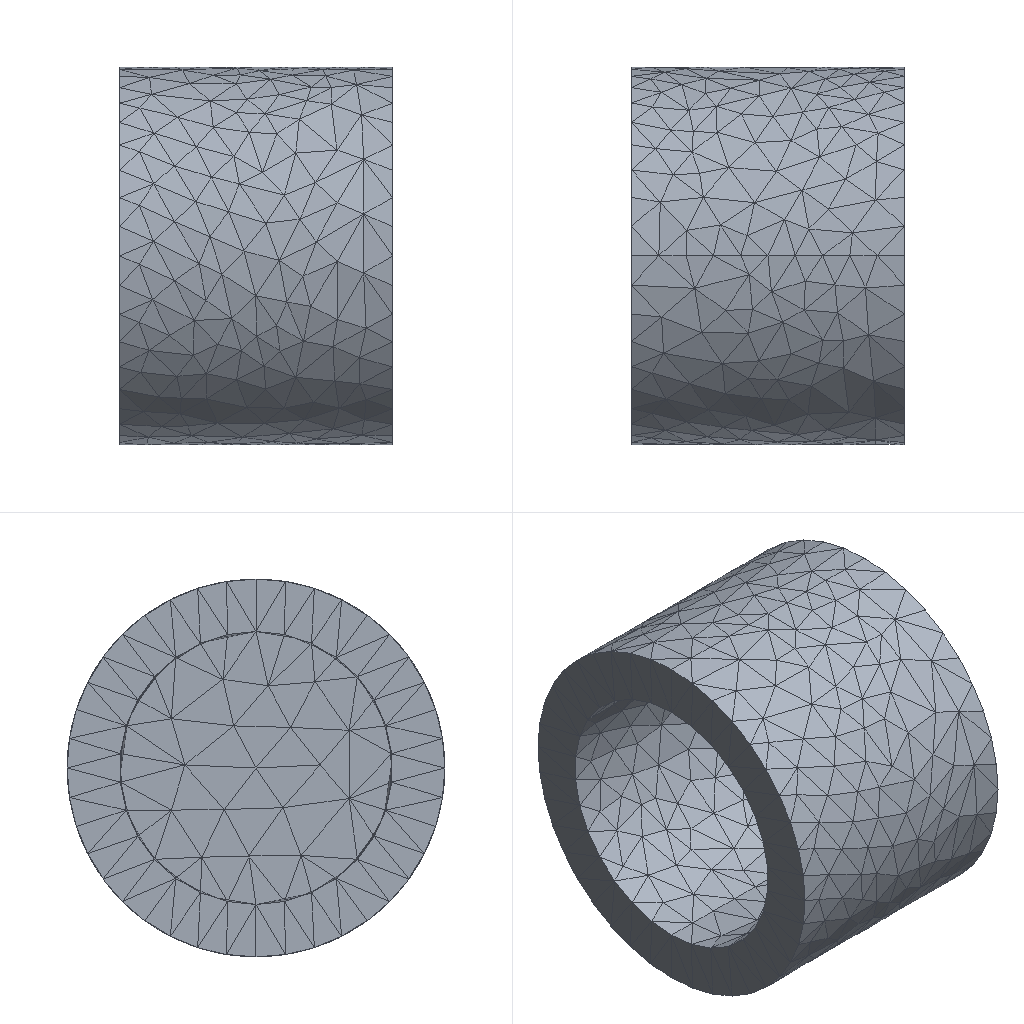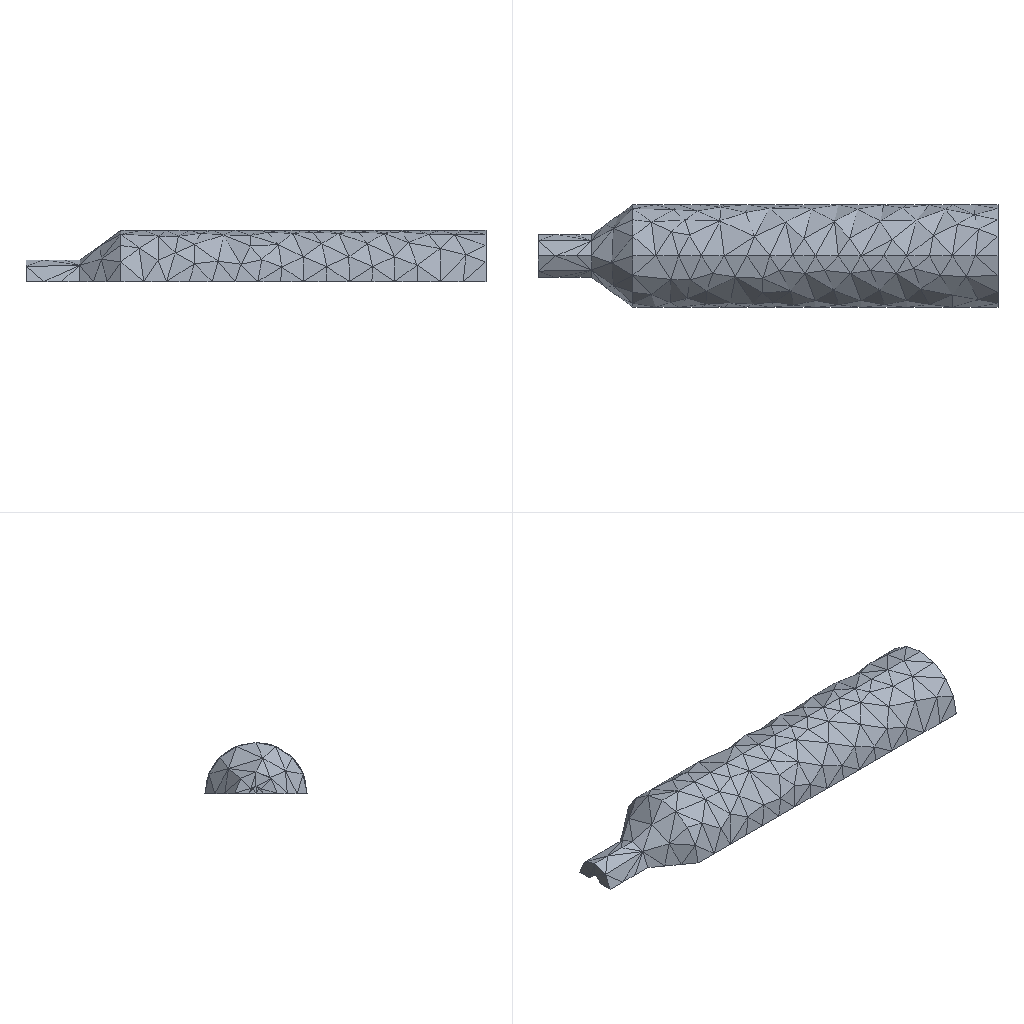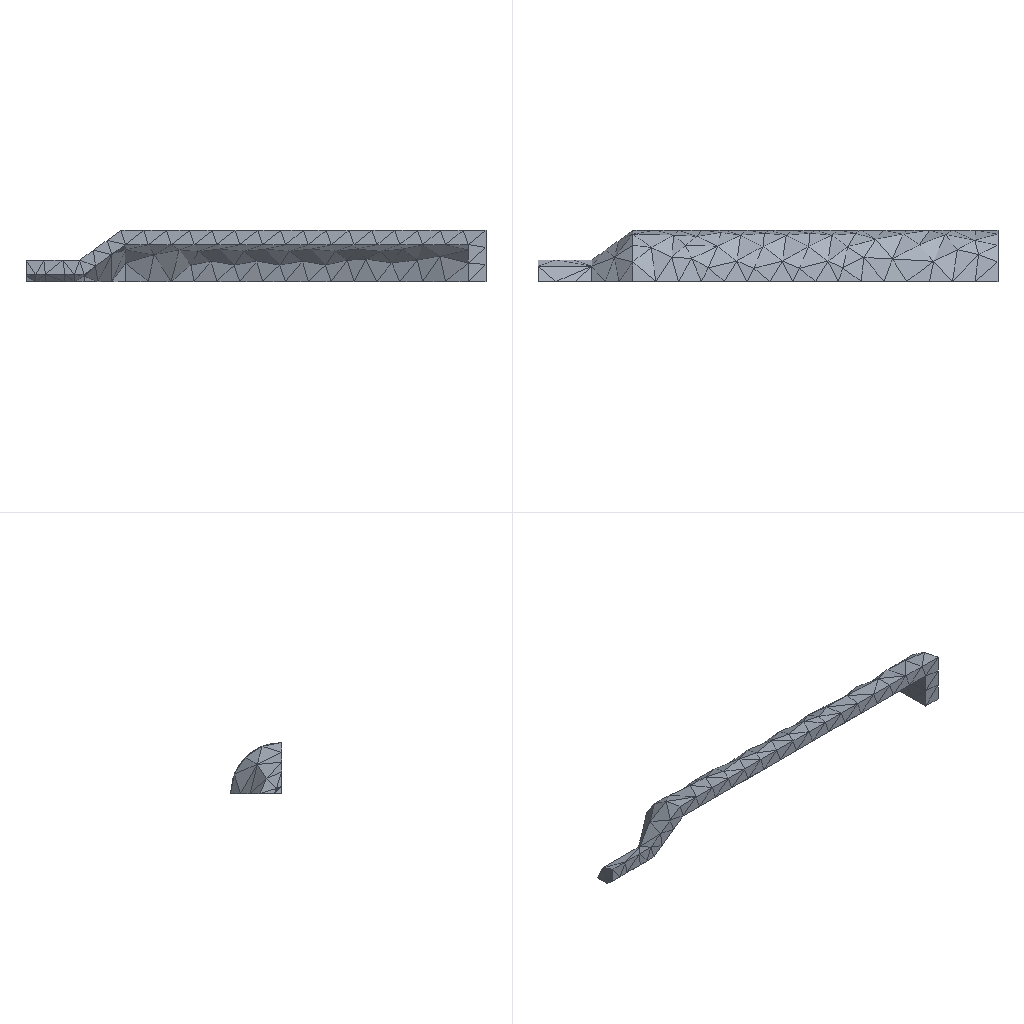Simulation study | ansys workbench
Set-up summary:
category,name,step,type,value,unit,region
solver,ansys_workbench
units,mm-N-s-tonne (MPa),,stated,"/units,MPA"
analysis,deck-1/LS1,,static
load_step,deck-1/LS1,deck-1/LS1,static,nsubst=1; time=1
analysis,deck-2/LS1,,static
load_step,deck-2/LS1,deck-2/LS1,static,nsubst=1; time=1
analysis,deck-3/LS1,,static
load_step,deck-3/LS1,deck-3/LS1,static,nsubst=1; time=1
mesh,deck-1.dat,,nodes,4771
mesh,deck-1.dat,,elements,3610
element_type,SOLID187,,,2632,,deck-1.dat
element_type,SURF154,,,978,,deck-1.dat
mesh,deck-2.dat,,nodes,1566
mesh,deck-2.dat,,elements,1070
element_type,SOLID187,,,706,,deck-2.dat
element_type,SURF154,,,364,,deck-2.dat
mesh,deck-3.dat,,nodes,897
mesh,deck-3.dat,,elements,561
element_type,SOLID187,,,373,,deck-3.dat
element_type,SURF154,,,188,,deck-3.dat
material,Structural Steel,,E,200000,tonne s^-2 mm^-1
material,Structural Steel,,nu,0.3
material,Structural Steel,,density,7.85e-09,tonne mm^-3
material,Structural Steel,,conductivity,60.5,tonne mm s^-3 C^-1
material,Structural Steel,,specific_heat,4.34e+08,mm^2 s^-2 C^-1
material,Structural Steel,,cte,1.2e-05,C^-1
material,Structural Steel,,permeability,10000
material,Structural Steel,,resistivity,0.00017,ohm mm
material,Structural Steel,,E,200000,tonne s^-2 mm^-1
material,Structural Steel,,nu,0.3
material,Structural Steel,,density,7.85e-09,tonne mm^-3
material,Structural Steel,,conductivity,60.5,tonne mm s^-3 C^-1
material,Structural Steel,,specific_heat,4.34e+08,mm^2 s^-2 C^-1
material,Structural Steel,,cte,1.2e-05,C^-1
material,Structural Steel,,permeability,10000
material,Structural Steel,,resistivity,0.00017,ohm mm
material,Structural Steel,,E,200000,tonne s^-2 mm^-1
material,Structural Steel,,nu,0.3
material,Structural Steel,,density,7.85e-09,tonne mm^-3
material,Structural Steel,,conductivity,60.5,tonne mm s^-3 C^-1
material,Structural Steel,,specific_heat,4.34e+08,mm^2 s^-2 C^-1
material,Structural Steel,,cte,1.2e-05,C^-1
material,Structural Steel,,permeability,10000
material,Structural Steel,,resistivity,0.00017,ohm mm
load,"Define Pressure Using Surface Effect Elements ""__""",deck-1/LS1,pressure,20,,SURF154 #2
load,"Define Pressure Using Surface Effect Elements ""__ 2""",deck-1/LS1,pressure,60,,SURF154 #3
load,"Define Pressure Using Surface Effect Elements ""__""",deck-2/LS1,pressure,20,,SURF154 #2
load,"Define Pressure Using Surface Effect Elements ""__ 2""",deck-2/LS1,pressure,60,,SURF154 #3
load,"Define Pressure Using Surface Effect Elements ""__""",deck-3/LS1,pressure,20,,SURF154 #2
load,"Define Pressure Using Surface Effect Elements ""__ 2""",deck-3/LS1,pressure,60,,SURF154 #3
bc,Fixed Supports,deck-1/model,fixed,[dofs=ALL],,_FIXEDSU
bc,Fixed Supports,deck-2/model,fixed,[dofs=ALL],,_FIXEDSU
bc,Fixed Supports,deck-3/model,fixed,[dofs=ALL],,_FIXEDSU
named_set,_FIXEDSU,,node,245
named_set,_FIXEDSU,,node,36
named_set,_FIXEDSU,,node,27
Results summary:
result,analyses[0].index,,,1
result,analyses[0].system,,,SYS
result,analyses[0].deck,,,deck-1.dat
result,analyses[0].solve_status,,,completed
result,analyses[0].analysis_type,,,static
result,analyses[0].physics,,,mechanical
result,analyses[0].unit_system,,,"NMM: mm, ton, N, s, mV, mA, degC"
result,analyses[0].n_sets,,,1
result,analyses[0].load_steps[0].set,set=1,,1
result,analyses[0].load_steps[0].time_or_freq,set=1,,1
result,analyses[0].load_steps[0].max_displacement_magnitude,set=1,,0.07354
result,analyses[0].load_steps[0].max_von_mises_nodal,set=1,,158.677
result,analyses[0].load_steps[0].reaction_force_sum_xyz[1],set=1,,8.00451e-08
result,analyses[0].load_steps[0].reaction_force_sum_xyz[2],set=1,,1.75338e-08
result,analyses[0].load_steps[0].reaction_force_sum_xyz[3],set=1,,-2.2319e-09
result,analyses[1].index,,,2
result,analyses[1].system,,,SYS-1
result,analyses[1].deck,,,deck-2.dat
result,analyses[1].solve_status,,,completed
result,analyses[1].analysis_type,,,static
result,analyses[1].physics,,,mechanical
result,analyses[1].unit_system,,,"NMM: mm, ton, N, s, mV, mA, degC"
result,analyses[1].n_sets,,,1
result,analyses[1].load_steps[0].set,set=1,,1
result,analyses[1].load_steps[0].time_or_freq,set=1,,1
result,analyses[1].load_steps[0].max_displacement_magnitude,set=1,,242.316
result,analyses[1].load_steps[0].max_von_mises_nodal,set=1,,9832.3
result,analyses[1].load_steps[0].reaction_force_sum_xyz[1],set=1,,-3.49525e-06
result,analyses[1].load_steps[0].reaction_force_sum_xyz[2],set=1,,1.4158e-05
result,analyses[1].load_steps[0].reaction_force_sum_xyz[3],set=1,,-6.17929e+06
result,analyses[2].index,,,3
result,analyses[2].system,,,SYS-2
result,analyses[2].deck,,,deck-3.dat
result,analyses[2].solve_status,,,completed
result,analyses[2].analysis_type,,,static
result,analyses[2].physics,,,mechanical
result,analyses[2].unit_system,,,"NMM: mm, ton, N, s, mV, mA, degC"
result,analyses[2].n_sets,,,1
result,analyses[2].load_steps[0].set,set=1,,1
result,analyses[2].load_steps[0].time_or_freq,set=1,,1
result,analyses[2].load_steps[0].max_displacement_magnitude,set=1,,2139.88
result,analyses[2].load_steps[0].max_von_mises_nodal,set=1,,42178.3
result,analyses[2].load_steps[0].reaction_force_sum_xyz[1],set=1,,-0.001879
result,analyses[2].load_steps[0].reaction_force_sum_xyz[2],set=1,,-3.08965e+06
result,analyses[2].load_steps[0].reaction_force_sum_xyz[3],set=1,,-3.08965e+06